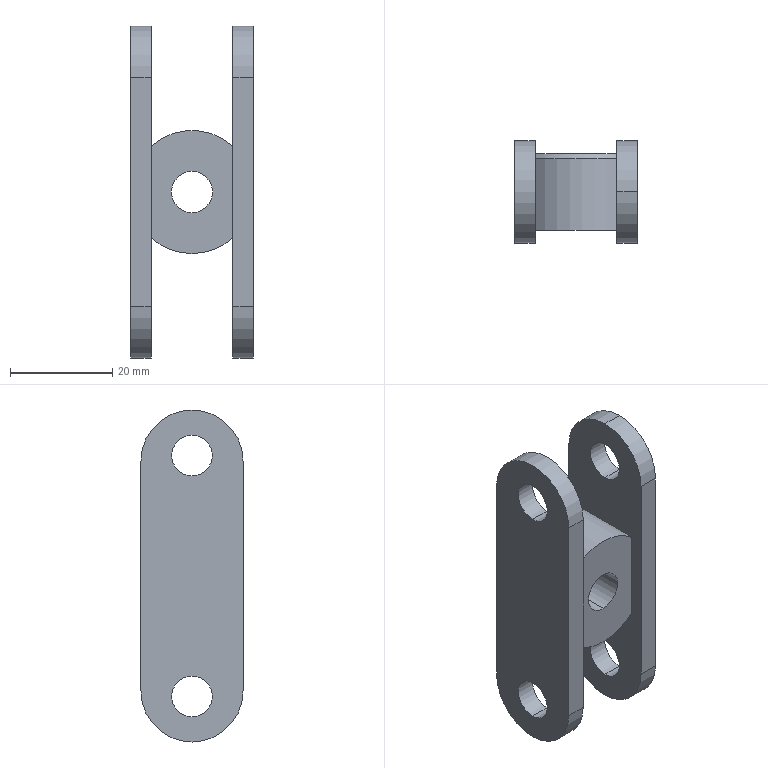Part | SolidWorks | features ICE 2, Chamfer 1, Extrusion 1, MirrorPattern 1 | 1 solid | 32 faces | box 24 x 20 x 65 mm | volume 13444 mm3 | cylinder 19 | plane 10 | cone 3 | commonest cylinder face diameters 8 x8 20 x6 24.1 x3 8.1 x2
STEP:
#1=CARTESIAN_POINT('',(-12.,7.5,27.58));
#2=VERTEX_POINT('',#1);
#3=CARTESIAN_POINT('',(-12.,7.5,19.58));
#4=VERTEX_POINT('',#3);
#5=CARTESIAN_POINT('',(-12.,7.5,23.58));
#6=DIRECTION('',(1.,0.,0.));
#7=DIRECTION('',(0.,0.,1.));
#8=AXIS2_PLACEMENT_3D('',#5,#6,#7);
#9=CIRCLE('',#8,4.);
#10=EDGE_CURVE('',#2,#4,#9,.T.);
#11=ORIENTED_EDGE('',*,*,#10,.F.);
#12=CARTESIAN_POINT('',(-8.,7.5,27.58));
#13=VERTEX_POINT('',#12);
#14=CARTESIAN_POINT('',(-12.,7.5,27.58));
#15=DIRECTION('',(1.,0.,0.));
#16=VECTOR('',#15,1000.);
#17=LINE('',#14,#16);
#18=EDGE_CURVE('',#2,#13,#17,.T.);
#19=ORIENTED_EDGE('',*,*,#18,.T.);
#20=CARTESIAN_POINT('',(-8.,7.5,19.58));
#21=VERTEX_POINT('',#20);
#22=CARTESIAN_POINT('',(-8.,7.5,23.58));
#23=DIRECTION('',(1.,0.,0.));
#24=DIRECTION('',(0.,0.,1.));
#25=AXIS2_PLACEMENT_3D('',#22,#23,#24);
#26=CIRCLE('',#25,4.);
#27=EDGE_CURVE('',#13,#21,#26,.T.);
#28=ORIENTED_EDGE('',*,*,#27,.T.);
#29=CARTESIAN_POINT('',(-12.,7.5,19.58));
#30=DIRECTION('',(1.,0.,0.));
#31=VECTOR('',#30,1000.);
#32=LINE('',#29,#31);
#33=EDGE_CURVE('',#4,#21,#32,.T.);
#34=ORIENTED_EDGE('',*,*,#33,.F.);
#35=EDGE_LOOP('',(#11,#19,#28,#34));
#36=FACE_OUTER_BOUND('',#35,.T.);
#37=CARTESIAN_POINT('',(-12.,7.5,23.58));
#38=DIRECTION('',(1.,0.,0.));
#39=DIRECTION('',(0.,0.,-1.));
#40=AXIS2_PLACEMENT_3D('',#37,#38,#39);
#41=CYLINDRICAL_SURFACE('',#40,4.);
#42=ADVANCED_FACE('',(#36),#41,.F.);
#43=CARTESIAN_POINT('',(-12.,7.5,-19.58));
#44=VERTEX_POINT('',#43);
#45=CARTESIAN_POINT('',(-12.,7.5,-27.58));
#46=VERTEX_POINT('',#45);
#47=CARTESIAN_POINT('',(-12.,7.5,-23.58));
#48=DIRECTION('',(1.,0.,0.));
#49=DIRECTION('',(0.,0.,-1.));
#50=AXIS2_PLACEMENT_3D('',#47,#48,#49);
#51=CIRCLE('',#50,4.);
#52=EDGE_CURVE('',#44,#46,#51,.T.);
#53=ORIENTED_EDGE('',*,*,#52,.F.);
#54=CARTESIAN_POINT('',(-8.,7.5,-19.58));
#55=VERTEX_POINT('',#54);
#56=CARTESIAN_POINT('',(-12.,7.5,-19.58));
#57=DIRECTION('',(1.,0.,0.));
#58=VECTOR('',#57,1000.);
#59=LINE('',#56,#58);
#60=EDGE_CURVE('',#44,#55,#59,.T.);
#61=ORIENTED_EDGE('',*,*,#60,.T.);
#62=CARTESIAN_POINT('',(-8.,7.5,-27.58));
#63=VERTEX_POINT('',#62);
#64=CARTESIAN_POINT('',(-8.,7.5,-23.58));
#65=DIRECTION('',(1.,0.,0.));
#66=DIRECTION('',(0.,0.,-1.));
#67=AXIS2_PLACEMENT_3D('',#64,#65,#66);
#68=CIRCLE('',#67,4.);
#69=EDGE_CURVE('',#55,#63,#68,.T.);
#70=ORIENTED_EDGE('',*,*,#69,.T.);
#71=CARTESIAN_POINT('',(-12.,7.5,-27.58));
#72=DIRECTION('',(1.,0.,0.));
#73=VECTOR('',#72,1000.);
#74=LINE('',#71,#73);
#75=EDGE_CURVE('',#46,#63,#74,.T.);
#76=ORIENTED_EDGE('',*,*,#75,.F.);
#77=EDGE_LOOP('',(#53,#61,#70,#76));
#78=FACE_OUTER_BOUND('',#77,.T.);
#79=CARTESIAN_POINT('',(-12.,7.5,-23.58));
#80=DIRECTION('',(1.,0.,0.));
#81=DIRECTION('',(0.,0.,-1.));
#82=AXIS2_PLACEMENT_3D('',#79,#80,#81);
#83=CYLINDRICAL_SURFACE('',#82,4.);
#84=ADVANCED_FACE('',(#78),#83,.F.);
#85=CARTESIAN_POINT('',(-12.,-2.5,-22.5));
#86=VERTEX_POINT('',#85);
#87=CARTESIAN_POINT('',(-12.,7.5,-32.5));
#88=VERTEX_POINT('',#87);
#89=CARTESIAN_POINT('',(-12.,7.5,-22.5));
#90=DIRECTION('',(1.,0.,0.));
#91=DIRECTION('',(0.,0.,-1.));
#92=AXIS2_PLACEMENT_3D('',#89,#90,#91);
#93=CIRCLE('',#92,10.);
#94=EDGE_CURVE('',#86,#88,#93,.T.);
#95=ORIENTED_EDGE('',*,*,#94,.T.);
#96=CARTESIAN_POINT('',(-8.,7.5,-32.5));
#97=VERTEX_POINT('',#96);
#98=CARTESIAN_POINT('',(-12.,7.5,-32.5));
#99=DIRECTION('',(1.,0.,0.));
#100=VECTOR('',#99,1000.);
#101=LINE('',#98,#100);
#102=EDGE_CURVE('',#88,#97,#101,.T.);
#103=ORIENTED_EDGE('',*,*,#102,.T.);
#104=CARTESIAN_POINT('',(-8.,-2.5,-22.5));
#105=VERTEX_POINT('',#104);
#106=CARTESIAN_POINT('',(-8.,7.5,-22.5));
#107=DIRECTION('',(1.,0.,0.));
#108=DIRECTION('',(0.,0.,-1.));
#109=AXIS2_PLACEMENT_3D('',#106,#107,#108);
#110=CIRCLE('',#109,10.);
#111=EDGE_CURVE('',#105,#97,#110,.T.);
#112=ORIENTED_EDGE('',*,*,#111,.F.);
#113=CARTESIAN_POINT('',(-12.,-2.5,-22.5));
#114=DIRECTION('',(1.,0.,0.));
#115=VECTOR('',#114,1000.);
#116=LINE('',#113,#115);
#117=EDGE_CURVE('',#86,#105,#116,.T.);
#118=ORIENTED_EDGE('',*,*,#117,.F.);
#119=EDGE_LOOP('',(#95,#103,#112,#118));
#120=FACE_OUTER_BOUND('',#119,.T.);
#121=CARTESIAN_POINT('',(-12.,7.5,-22.5));
#122=DIRECTION('',(1.,0.,0.));
#123=DIRECTION('',(0.,0.,-1.));
#124=AXIS2_PLACEMENT_3D('',#121,#122,#123);
#125=CYLINDRICAL_SURFACE('',#124,10.);
#126=ADVANCED_FACE('',(#120),#125,.T.);
#127=CARTESIAN_POINT('',(12.,7.5,27.58));
#128=VERTEX_POINT('',#127);
#129=CARTESIAN_POINT('',(12.,7.5,19.58));
#130=VERTEX_POINT('',#129);
#131=CARTESIAN_POINT('',(12.,7.5,23.58));
#132=DIRECTION('',(1.,0.,0.));
#133=DIRECTION('',(0.,0.,1.));
#134=AXIS2_PLACEMENT_3D('',#131,#132,#133);
#135=CIRCLE('',#134,4.);
#136=EDGE_CURVE('',#128,#130,#135,.T.);
#137=ORIENTED_EDGE('',*,*,#136,.T.);
#138=CARTESIAN_POINT('',(8.,7.5,19.58));
#139=VERTEX_POINT('',#138);
#140=CARTESIAN_POINT('',(12.,7.5,19.58));
#141=DIRECTION('',(-1.,0.,0.));
#142=VECTOR('',#141,1000.);
#143=LINE('',#140,#142);
#144=EDGE_CURVE('',#130,#139,#143,.T.);
#145=ORIENTED_EDGE('',*,*,#144,.T.);
#146=CARTESIAN_POINT('',(8.,7.5,27.58));
#147=VERTEX_POINT('',#146);
#148=CARTESIAN_POINT('',(8.,7.5,23.58));
#149=DIRECTION('',(1.,0.,0.));
#150=DIRECTION('',(0.,0.,1.));
#151=AXIS2_PLACEMENT_3D('',#148,#149,#150);
#152=CIRCLE('',#151,4.);
#153=EDGE_CURVE('',#147,#139,#152,.T.);
#154=ORIENTED_EDGE('',*,*,#153,.F.);
#155=CARTESIAN_POINT('',(12.,7.5,27.58));
#156=DIRECTION('',(-1.,0.,0.));
#157=VECTOR('',#156,1000.);
#158=LINE('',#155,#157);
#159=EDGE_CURVE('',#128,#147,#158,.T.);
#160=ORIENTED_EDGE('',*,*,#159,.F.);
#161=EDGE_LOOP('',(#137,#145,#154,#160));
#162=FACE_OUTER_BOUND('',#161,.T.);
#163=CARTESIAN_POINT('',(12.,7.5,23.58));
#164=DIRECTION('',(-1.,0.,0.));
#165=DIRECTION('',(0.,0.,1.));
#166=AXIS2_PLACEMENT_3D('',#163,#164,#165);
#167=CYLINDRICAL_SURFACE('',#166,4.);
#168=ADVANCED_FACE('',(#162),#167,.F.);
#169=CARTESIAN_POINT('',(12.,7.5,-19.58));
#170=VERTEX_POINT('',#169);
#171=CARTESIAN_POINT('',(12.,7.5,-27.58));
#172=VERTEX_POINT('',#171);
#173=CARTESIAN_POINT('',(12.,7.5,-23.58));
#174=DIRECTION('',(1.,0.,0.));
#175=DIRECTION('',(0.,0.,-1.));
#176=AXIS2_PLACEMENT_3D('',#173,#174,#175);
#177=CIRCLE('',#176,4.);
#178=EDGE_CURVE('',#170,#172,#177,.T.);
#179=ORIENTED_EDGE('',*,*,#178,.T.);
#180=CARTESIAN_POINT('',(8.,7.5,-27.58));
#181=VERTEX_POINT('',#180);
#182=CARTESIAN_POINT('',(12.,7.5,-27.58));
#183=DIRECTION('',(-1.,0.,0.));
#184=VECTOR('',#183,1000.);
#185=LINE('',#182,#184);
#186=EDGE_CURVE('',#172,#181,#185,.T.);
#187=ORIENTED_EDGE('',*,*,#186,.T.);
#188=CARTESIAN_POINT('',(8.,7.5,-19.58));
#189=VERTEX_POINT('',#188);
#190=CARTESIAN_POINT('',(8.,7.5,-23.58));
#191=DIRECTION('',(1.,0.,0.));
#192=DIRECTION('',(0.,0.,-1.));
#193=AXIS2_PLACEMENT_3D('',#190,#191,#192);
#194=CIRCLE('',#193,4.);
#195=EDGE_CURVE('',#189,#181,#194,.T.);
#196=ORIENTED_EDGE('',*,*,#195,.F.);
#197=CARTESIAN_POINT('',(12.,7.5,-19.58));
#198=DIRECTION('',(-1.,0.,0.));
#199=VECTOR('',#198,1000.);
#200=LINE('',#197,#199);
#201=EDGE_CURVE('',#170,#189,#200,.T.);
#202=ORIENTED_EDGE('',*,*,#201,.F.);
#203=EDGE_LOOP('',(#179,#187,#196,#202));
#204=FACE_OUTER_BOUND('',#203,.T.);
#205=CARTESIAN_POINT('',(12.,7.5,-23.58));
#206=DIRECTION('',(-1.,0.,0.));
#207=DIRECTION('',(0.,0.,1.));
#208=AXIS2_PLACEMENT_3D('',#205,#206,#207);
#209=CYLINDRICAL_SURFACE('',#208,4.);
#210=ADVANCED_FACE('',(#204),#209,.F.);
#211=CARTESIAN_POINT('',(12.,7.5,32.5));
#212=VERTEX_POINT('',#211);
#213=CARTESIAN_POINT('',(12.,-2.5,22.5));
#214=VERTEX_POINT('',#213);
#215=CARTESIAN_POINT('',(12.,7.5,22.5));
#216=DIRECTION('',(1.,0.,0.));
#217=DIRECTION('',(0.,0.,-1.));
#218=AXIS2_PLACEMENT_3D('',#215,#216,#217);
#219=CIRCLE('',#218,10.);
#220=EDGE_CURVE('',#212,#214,#219,.T.);
#221=ORIENTED_EDGE('',*,*,#220,.F.);
#222=CARTESIAN_POINT('',(8.,7.5,32.5));
#223=VERTEX_POINT('',#222);
#224=CARTESIAN_POINT('',(12.,7.5,32.5));
#225=DIRECTION('',(-1.,0.,0.));
#226=VECTOR('',#225,1000.);
#227=LINE('',#224,#226);
#228=EDGE_CURVE('',#212,#223,#227,.T.);
#229=ORIENTED_EDGE('',*,*,#228,.T.);
#230=CARTESIAN_POINT('',(8.,-2.5,22.5));
#231=VERTEX_POINT('',#230);
#232=CARTESIAN_POINT('',(8.,7.5,22.5));
#233=DIRECTION('',(1.,0.,0.));
#234=DIRECTION('',(0.,0.,-1.));
#235=AXIS2_PLACEMENT_3D('',#232,#233,#234);
#236=CIRCLE('',#235,10.);
#237=EDGE_CURVE('',#223,#231,#236,.T.);
#238=ORIENTED_EDGE('',*,*,#237,.T.);
#239=CARTESIAN_POINT('',(12.,-2.5,22.5));
#240=DIRECTION('',(-1.,0.,0.));
#241=VECTOR('',#240,1000.);
#242=LINE('',#239,#241);
#243=EDGE_CURVE('',#214,#231,#242,.T.);
#244=ORIENTED_EDGE('',*,*,#243,.F.);
#245=EDGE_LOOP('',(#221,#229,#238,#244));
#246=FACE_OUTER_BOUND('',#245,.T.);
#247=CARTESIAN_POINT('',(12.,7.5,22.5));
#248=DIRECTION('',(-1.,0.,0.));
#249=DIRECTION('',(0.,0.,1.));
#250=AXIS2_PLACEMENT_3D('',#247,#248,#249);
#251=CYLINDRICAL_SURFACE('',#250,10.);
#252=ADVANCED_FACE('',(#246),#251,.T.);
#253=CARTESIAN_POINT('',(0.,15.,-4.05));
#254=VERTEX_POINT('',#253);
#255=CARTESIAN_POINT('',(0.,15.,4.05));
#256=VERTEX_POINT('',#255);
#257=CARTESIAN_POINT('',(0.,15.,0.));
#258=DIRECTION('',(0.,1.,0.));
#259=DIRECTION('',(0.,0.,1.));
#260=AXIS2_PLACEMENT_3D('',#257,#258,#259);
#261=CIRCLE('',#260,4.05);
#262=EDGE_CURVE('',#254,#256,#261,.T.);
#263=ORIENTED_EDGE('',*,*,#262,.T.);
#264=CARTESIAN_POINT('',(0.,0.,4.05));
#265=VERTEX_POINT('',#264);
#266=CARTESIAN_POINT('',(0.,15.,4.05));
#267=DIRECTION('',(0.,-1.,0.));
#268=VECTOR('',#267,1000.);
#269=LINE('',#266,#268);
#270=EDGE_CURVE('',#256,#265,#269,.T.);
#271=ORIENTED_EDGE('',*,*,#270,.T.);
#272=CARTESIAN_POINT('',(0.,0.,-4.05));
#273=VERTEX_POINT('',#272);
#274=CARTESIAN_POINT('',(0.,0.,0.));
#275=DIRECTION('',(0.,1.,0.));
#276=DIRECTION('',(0.,0.,1.));
#277=AXIS2_PLACEMENT_3D('',#274,#275,#276);
#278=CIRCLE('',#277,4.05);
#279=EDGE_CURVE('',#273,#265,#278,.T.);
#280=ORIENTED_EDGE('',*,*,#279,.F.);
#281=CARTESIAN_POINT('',(0.,15.,-4.05));
#282=DIRECTION('',(0.,-1.,0.));
#283=VECTOR('',#282,1000.);
#284=LINE('',#281,#283);
#285=EDGE_CURVE('',#254,#273,#284,.T.);
#286=ORIENTED_EDGE('',*,*,#285,.F.);
#287=EDGE_LOOP('',(#263,#271,#280,#286));
#288=FACE_OUTER_BOUND('',#287,.T.);
#289=CARTESIAN_POINT('',(0.,15.,0.));
#290=DIRECTION('',(0.,-1.,0.));
#291=DIRECTION('',(0.,0.,-1.));
#292=AXIS2_PLACEMENT_3D('',#289,#290,#291);
#293=CYLINDRICAL_SURFACE('',#292,4.05);
#294=ADVANCED_FACE('',(#288),#293,.F.);
#295=CARTESIAN_POINT('',(0.,15.,-11.05));
#296=VERTEX_POINT('',#295);
#297=CARTESIAN_POINT('',(-8.,15.,-7.622));
#298=VERTEX_POINT('',#297);
#299=CARTESIAN_POINT('',(0.,15.,0.));
#300=DIRECTION('',(0.,1.,0.));
#301=DIRECTION('',(0.,0.,1.));
#302=AXIS2_PLACEMENT_3D('',#299,#300,#301);
#303=CIRCLE('',#302,11.05);
#304=EDGE_CURVE('',#296,#298,#303,.T.);
#305=ORIENTED_EDGE('',*,*,#304,.F.);
#306=CARTESIAN_POINT('',(0.,14.,-12.05));
#307=VERTEX_POINT('',#306);
#308=CARTESIAN_POINT('',(0.,15.,-11.05));
#309=DIRECTION('',(0.,-0.7071,-0.7071));
#310=VECTOR('',#309,1000.);
#311=LINE('',#308,#310);
#312=EDGE_CURVE('',#296,#307,#311,.T.);
#313=ORIENTED_EDGE('',*,*,#312,.T.);
#314=CARTESIAN_POINT('',(-8.,14.,-9.011));
#315=VERTEX_POINT('',#314);
#316=CARTESIAN_POINT('',(0.,14.,0.));
#317=DIRECTION('',(0.,-1.,0.));
#318=DIRECTION('',(0.,0.,1.));
#319=AXIS2_PLACEMENT_3D('',#316,#317,#318);
#320=CIRCLE('',#319,12.05);
#321=EDGE_CURVE('',#315,#307,#320,.T.);
#322=ORIENTED_EDGE('',*,*,#321,.F.);
#323=CARTESIAN_POINT('',(-8.,15.,-7.622));
#324=CARTESIAN_POINT('',(-8.,14.677,-8.091));
#325=CARTESIAN_POINT('',(-8.,14.342,-8.554));
#326=CARTESIAN_POINT('',(-8.,14.,-9.011));
#327=B_SPLINE_CURVE_WITH_KNOTS('',3,(#323,#324,#325,#326),.UNSPECIFIED.,.F.,.F.,(4,4),(0.0402,0.04192),.UNSPECIFIED.);
#328=EDGE_CURVE('',#298,#315,#327,.T.);
#329=ORIENTED_EDGE('',*,*,#328,.F.);
#330=EDGE_LOOP('',(#305,#313,#322,#329));
#331=FACE_OUTER_BOUND('',#330,.T.);
#332=CARTESIAN_POINT('',(0.,15.,0.));
#333=DIRECTION('',(0.,-1.,0.));
#334=DIRECTION('',(0.,0.,-1.));
#335=AXIS2_PLACEMENT_3D('',#332,#333,#334);
#336=CONICAL_SURFACE('',#335,11.05,0.7854);
#337=ADVANCED_FACE('',(#331),#336,.T.);
#338=ORIENTED_EDGE('',*,*,#321,.T.);
#339=CARTESIAN_POINT('',(0.,0.,-12.05));
#340=VERTEX_POINT('',#339);
#341=CARTESIAN_POINT('',(0.,15.,-12.05));
#342=DIRECTION('',(0.,-1.,0.));
#343=VECTOR('',#342,1000.);
#344=LINE('',#341,#343);
#345=EDGE_CURVE('',#307,#340,#344,.T.);
#346=ORIENTED_EDGE('',*,*,#345,.T.);
#347=CARTESIAN_POINT('',(-8.,0.,-9.011));
#348=VERTEX_POINT('',#347);
#349=CARTESIAN_POINT('',(0.,0.,0.));
#350=DIRECTION('',(0.,1.,0.));
#351=DIRECTION('',(0.,0.,1.));
#352=AXIS2_PLACEMENT_3D('',#349,#350,#351);
#353=CIRCLE('',#352,12.05);
#354=EDGE_CURVE('',#340,#348,#353,.T.);
#355=ORIENTED_EDGE('',*,*,#354,.T.);
#356=CARTESIAN_POINT('',(-8.,15.,-9.011));
#357=DIRECTION('',(0.,1.,0.));
#358=VECTOR('',#357,1000.);
#359=LINE('',#356,#358);
#360=EDGE_CURVE('',#348,#315,#359,.T.);
#361=ORIENTED_EDGE('',*,*,#360,.T.);
#362=EDGE_LOOP('',(#338,#346,#355,#361));
#363=FACE_OUTER_BOUND('',#362,.T.);
#364=CARTESIAN_POINT('',(0.,15.,0.));
#365=DIRECTION('',(0.,-1.,0.));
#366=DIRECTION('',(0.,0.,-1.));
#367=AXIS2_PLACEMENT_3D('',#364,#365,#366);
#368=CYLINDRICAL_SURFACE('',#367,12.05);
#369=ADVANCED_FACE('',(#363),#368,.T.);
#370=ORIENTED_EDGE('',*,*,#345,.F.);
#371=CARTESIAN_POINT('',(8.,14.,-9.011));
#372=VERTEX_POINT('',#371);
#373=CARTESIAN_POINT('',(0.,14.,0.));
#374=DIRECTION('',(0.,-1.,0.));
#375=DIRECTION('',(0.,0.,1.));
#376=AXIS2_PLACEMENT_3D('',#373,#374,#375);
#377=CIRCLE('',#376,12.05);
#378=EDGE_CURVE('',#307,#372,#377,.T.);
#379=ORIENTED_EDGE('',*,*,#378,.T.);
#380=CARTESIAN_POINT('',(8.,0.,-9.011));
#381=VERTEX_POINT('',#380);
#382=CARTESIAN_POINT('',(8.,15.,-9.011));
#383=DIRECTION('',(0.,1.,0.));
#384=VECTOR('',#383,1000.);
#385=LINE('',#382,#384);
#386=EDGE_CURVE('',#381,#372,#385,.T.);
#387=ORIENTED_EDGE('',*,*,#386,.F.);
#388=CARTESIAN_POINT('',(0.,0.,0.));
#389=DIRECTION('',(0.,1.,0.));
#390=DIRECTION('',(0.,0.,1.));
#391=AXIS2_PLACEMENT_3D('',#388,#389,#390);
#392=CIRCLE('',#391,12.05);
#393=EDGE_CURVE('',#381,#340,#392,.T.);
#394=ORIENTED_EDGE('',*,*,#393,.T.);
#395=EDGE_LOOP('',(#370,#379,#387,#394));
#396=FACE_OUTER_BOUND('',#395,.T.);
#397=CARTESIAN_POINT('',(0.,15.,0.));
#398=DIRECTION('',(0.,-1.,0.));
#399=DIRECTION('',(0.,0.,-1.));
#400=AXIS2_PLACEMENT_3D('',#397,#398,#399);
#401=CYLINDRICAL_SURFACE('',#400,12.05);
#402=ADVANCED_FACE('',(#396),#401,.T.);
#403=ORIENTED_EDGE('',*,*,#312,.F.);
#404=CARTESIAN_POINT('',(8.,15.,-7.622));
#405=VERTEX_POINT('',#404);
#406=CARTESIAN_POINT('',(0.,15.,0.));
#407=DIRECTION('',(0.,1.,0.));
#408=DIRECTION('',(0.,0.,1.));
#409=AXIS2_PLACEMENT_3D('',#406,#407,#408);
#410=CIRCLE('',#409,11.05);
#411=EDGE_CURVE('',#405,#296,#410,.T.);
#412=ORIENTED_EDGE('',*,*,#411,.F.);
#413=CARTESIAN_POINT('',(8.,15.,-7.622));
#414=CARTESIAN_POINT('',(8.,14.677,-8.091));
#415=CARTESIAN_POINT('',(8.,14.342,-8.554));
#416=CARTESIAN_POINT('',(8.,14.,-9.011));
#417=B_SPLINE_CURVE_WITH_KNOTS('',3,(#413,#414,#415,#416),.UNSPECIFIED.,.F.,.F.,(4,4),(0.0402,0.04192),.UNSPECIFIED.);
#418=EDGE_CURVE('',#405,#372,#417,.T.);
#419=ORIENTED_EDGE('',*,*,#418,.T.);
#420=ORIENTED_EDGE('',*,*,#378,.F.);
#421=EDGE_LOOP('',(#403,#412,#419,#420));
#422=FACE_OUTER_BOUND('',#421,.T.);
#423=CARTESIAN_POINT('',(0.,15.,0.));
#424=DIRECTION('',(0.,-1.,0.));
#425=DIRECTION('',(0.,0.,-1.));
#426=AXIS2_PLACEMENT_3D('',#423,#424,#425);
#427=CONICAL_SURFACE('',#426,11.05,0.7854);
#428=ADVANCED_FACE('',(#422),#427,.T.);
#429=CARTESIAN_POINT('',(8.,15.,7.622));
#430=VERTEX_POINT('',#429);
#431=CARTESIAN_POINT('',(8.,15.,-18.778));
#432=DIRECTION('',(0.,0.,1.));
#433=VECTOR('',#432,1000.);
#434=LINE('',#431,#433);
#435=EDGE_CURVE('',#405,#430,#434,.T.);
#436=ORIENTED_EDGE('',*,*,#435,.F.);
#437=ORIENTED_EDGE('',*,*,#411,.T.);
#438=ORIENTED_EDGE('',*,*,#304,.T.);
#439=CARTESIAN_POINT('',(-8.,15.,7.622));
#440=VERTEX_POINT('',#439);
#441=CARTESIAN_POINT('',(-8.,15.,-18.778));
#442=DIRECTION('',(0.,0.,1.));
#443=VECTOR('',#442,1000.);
#444=LINE('',#441,#443);
#445=EDGE_CURVE('',#298,#440,#444,.T.);
#446=ORIENTED_EDGE('',*,*,#445,.T.);
#447=CARTESIAN_POINT('',(0.,15.,0.));
#448=DIRECTION('',(0.,1.,0.));
#449=DIRECTION('',(0.,0.,1.));
#450=AXIS2_PLACEMENT_3D('',#447,#448,#449);
#451=CIRCLE('',#450,11.05);
#452=EDGE_CURVE('',#440,#430,#451,.T.);
#453=ORIENTED_EDGE('',*,*,#452,.T.);
#454=EDGE_LOOP('',(#436,#437,#438,#446,#453));
#455=FACE_OUTER_BOUND('',#454,.T.);
#456=ORIENTED_EDGE('',*,*,#262,.F.);
#457=CARTESIAN_POINT('',(0.,15.,0.));
#458=DIRECTION('',(0.,1.,0.));
#459=DIRECTION('',(0.,0.,1.));
#460=AXIS2_PLACEMENT_3D('',#457,#458,#459);
#461=CIRCLE('',#460,4.05);
#462=EDGE_CURVE('',#256,#254,#461,.T.);
#463=ORIENTED_EDGE('',*,*,#462,.F.);
#464=EDGE_LOOP('',(#456,#463));
#465=FACE_BOUND('',#464,.T.);
#466=CARTESIAN_POINT('',(0.,15.,0.));
#467=DIRECTION('',(0.,1.,0.));
#468=DIRECTION('',(0.,0.,1.));
#469=AXIS2_PLACEMENT_3D('',#466,#467,#468);
#470=PLANE('',#469);
#471=ADVANCED_FACE('',(#455,#465),#470,.T.);
#472=ORIENTED_EDGE('',*,*,#279,.T.);
#473=CARTESIAN_POINT('',(0.,0.,0.));
#474=DIRECTION('',(0.,1.,0.));
#475=DIRECTION('',(0.,0.,1.));
#476=AXIS2_PLACEMENT_3D('',#473,#474,#475);
#477=CIRCLE('',#476,4.05);
#478=EDGE_CURVE('',#265,#273,#477,.T.);
#479=ORIENTED_EDGE('',*,*,#478,.T.);
#480=EDGE_LOOP('',(#472,#479));
#481=FACE_BOUND('',#480,.T.);
#482=ORIENTED_EDGE('',*,*,#393,.F.);
#483=CARTESIAN_POINT('',(8.,0.,9.011));
#484=VERTEX_POINT('',#483);
#485=CARTESIAN_POINT('',(8.,0.,-18.778));
#486=DIRECTION('',(0.,0.,-1.));
#487=VECTOR('',#486,1000.);
#488=LINE('',#485,#487);
#489=EDGE_CURVE('',#484,#381,#488,.T.);
#490=ORIENTED_EDGE('',*,*,#489,.F.);
#491=CARTESIAN_POINT('',(-8.,0.,9.011));
#492=VERTEX_POINT('',#491);
#493=CARTESIAN_POINT('',(0.,0.,0.));
#494=DIRECTION('',(0.,1.,0.));
#495=DIRECTION('',(0.,0.,1.));
#496=AXIS2_PLACEMENT_3D('',#493,#494,#495);
#497=CIRCLE('',#496,12.05);
#498=EDGE_CURVE('',#492,#484,#497,.T.);
#499=ORIENTED_EDGE('',*,*,#498,.F.);
#500=CARTESIAN_POINT('',(-8.,0.,-18.778));
#501=DIRECTION('',(0.,0.,-1.));
#502=VECTOR('',#501,1000.);
#503=LINE('',#500,#502);
#504=EDGE_CURVE('',#492,#348,#503,.T.);
#505=ORIENTED_EDGE('',*,*,#504,.T.);
#506=ORIENTED_EDGE('',*,*,#354,.F.);
#507=EDGE_LOOP('',(#482,#490,#499,#505,#506));
#508=FACE_OUTER_BOUND('',#507,.T.);
#509=CARTESIAN_POINT('',(0.,0.,0.));
#510=DIRECTION('',(0.,1.,0.));
#511=DIRECTION('',(0.,0.,1.));
#512=AXIS2_PLACEMENT_3D('',#509,#510,#511);
#513=PLANE('',#512);
#514=ADVANCED_FACE('',(#481,#508),#513,.F.);
#515=ORIENTED_EDGE('',*,*,#498,.T.);
#516=CARTESIAN_POINT('',(8.,14.,9.011));
#517=VERTEX_POINT('',#516);
#518=CARTESIAN_POINT('',(8.,15.,9.011));
#519=DIRECTION('',(0.,-1.,0.));
#520=VECTOR('',#519,1000.);
#521=LINE('',#518,#520);
#522=EDGE_CURVE('',#517,#484,#521,.T.);
#523=ORIENTED_EDGE('',*,*,#522,.F.);
#524=CARTESIAN_POINT('',(-8.,14.,9.011));
#525=VERTEX_POINT('',#524);
#526=CARTESIAN_POINT('',(0.,14.,0.));
#527=DIRECTION('',(0.,-1.,0.));
#528=DIRECTION('',(0.,0.,1.));
#529=AXIS2_PLACEMENT_3D('',#526,#527,#528);
#530=CIRCLE('',#529,12.05);
#531=EDGE_CURVE('',#517,#525,#530,.T.);
#532=ORIENTED_EDGE('',*,*,#531,.T.);
#533=CARTESIAN_POINT('',(-8.,15.,9.011));
#534=DIRECTION('',(0.,-1.,0.));
#535=VECTOR('',#534,1000.);
#536=LINE('',#533,#535);
#537=EDGE_CURVE('',#525,#492,#536,.T.);
#538=ORIENTED_EDGE('',*,*,#537,.T.);
#539=EDGE_LOOP('',(#515,#523,#532,#538));
#540=FACE_OUTER_BOUND('',#539,.T.);
#541=CARTESIAN_POINT('',(0.,15.,0.));
#542=DIRECTION('',(0.,-1.,0.));
#543=DIRECTION('',(0.,0.,-1.));
#544=AXIS2_PLACEMENT_3D('',#541,#542,#543);
#545=CYLINDRICAL_SURFACE('',#544,12.05);
#546=ADVANCED_FACE('',(#540),#545,.T.);
#547=CARTESIAN_POINT('',(8.,14.,9.011));
#548=CARTESIAN_POINT('',(8.,14.341,8.555));
#549=CARTESIAN_POINT('',(8.,14.676,8.093));
#550=CARTESIAN_POINT('',(8.,15.,7.622));
#551=B_SPLINE_CURVE_WITH_KNOTS('',3,(#547,#548,#549,#550),.UNSPECIFIED.,.F.,.F.,(4,4),(0.02179,0.02351),.UNSPECIFIED.);
#552=EDGE_CURVE('',#517,#430,#551,.T.);
#553=ORIENTED_EDGE('',*,*,#552,.T.);
#554=ORIENTED_EDGE('',*,*,#452,.F.);
#555=CARTESIAN_POINT('',(-8.,14.,9.011));
#556=CARTESIAN_POINT('',(-8.,14.341,8.555));
#557=CARTESIAN_POINT('',(-8.,14.676,8.093));
#558=CARTESIAN_POINT('',(-8.,15.,7.622));
#559=B_SPLINE_CURVE_WITH_KNOTS('',3,(#555,#556,#557,#558),.UNSPECIFIED.,.F.,.F.,(4,4),(0.02179,0.02351),.UNSPECIFIED.);
#560=EDGE_CURVE('',#525,#440,#559,.T.);
#561=ORIENTED_EDGE('',*,*,#560,.F.);
#562=ORIENTED_EDGE('',*,*,#531,.F.);
#563=EDGE_LOOP('',(#553,#554,#561,#562));
#564=FACE_OUTER_BOUND('',#563,.T.);
#565=CARTESIAN_POINT('',(0.,15.,0.));
#566=DIRECTION('',(0.,-1.,0.));
#567=DIRECTION('',(0.,0.,-1.));
#568=AXIS2_PLACEMENT_3D('',#565,#566,#567);
#569=CONICAL_SURFACE('',#568,11.05,0.7854);
#570=ADVANCED_FACE('',(#564),#569,.T.);
#571=ORIENTED_EDGE('',*,*,#270,.F.);
#572=ORIENTED_EDGE('',*,*,#462,.T.);
#573=ORIENTED_EDGE('',*,*,#285,.T.);
#574=ORIENTED_EDGE('',*,*,#478,.F.);
#575=EDGE_LOOP('',(#571,#572,#573,#574));
#576=FACE_OUTER_BOUND('',#575,.T.);
#577=CARTESIAN_POINT('',(0.,15.,0.));
#578=DIRECTION('',(0.,-1.,0.));
#579=DIRECTION('',(0.,0.,-1.));
#580=AXIS2_PLACEMENT_3D('',#577,#578,#579);
#581=CYLINDRICAL_SURFACE('',#580,4.05);
#582=ADVANCED_FACE('',(#576),#581,.F.);
#583=CARTESIAN_POINT('',(8.,-2.5,-22.5));
#584=VERTEX_POINT('',#583);
#585=CARTESIAN_POINT('',(8.,17.5,-22.5));
#586=VERTEX_POINT('',#585);
#587=CARTESIAN_POINT('',(8.,7.5,-22.5));
#588=DIRECTION('',(1.,0.,0.));
#589=DIRECTION('',(0.,0.,-1.));
#590=AXIS2_PLACEMENT_3D('',#587,#588,#589);
#591=CIRCLE('',#590,10.);
#592=EDGE_CURVE('',#584,#586,#591,.T.);
#593=ORIENTED_EDGE('',*,*,#592,.F.);
#594=CARTESIAN_POINT('',(8.,-2.5,-22.5));
#595=DIRECTION('',(0.,0.,-1.));
#596=VECTOR('',#595,1000.);
#597=LINE('',#594,#596);
#598=EDGE_CURVE('',#231,#584,#597,.T.);
#599=ORIENTED_EDGE('',*,*,#598,.F.);
#600=ORIENTED_EDGE('',*,*,#237,.F.);
#601=CARTESIAN_POINT('',(8.,17.5,22.5));
#602=VERTEX_POINT('',#601);
#603=CARTESIAN_POINT('',(8.,7.5,22.5));
#604=DIRECTION('',(1.,0.,0.));
#605=DIRECTION('',(0.,0.,-1.));
#606=AXIS2_PLACEMENT_3D('',#603,#604,#605);
#607=CIRCLE('',#606,10.);
#608=EDGE_CURVE('',#602,#223,#607,.T.);
#609=ORIENTED_EDGE('',*,*,#608,.F.);
#610=CARTESIAN_POINT('',(8.,17.5,-22.5));
#611=DIRECTION('',(0.,0.,1.));
#612=VECTOR('',#611,1000.);
#613=LINE('',#610,#612);
#614=EDGE_CURVE('',#586,#602,#613,.T.);
#615=ORIENTED_EDGE('',*,*,#614,.F.);
#616=EDGE_LOOP('',(#593,#599,#600,#609,#615));
#617=FACE_OUTER_BOUND('',#616,.T.);
#618=ORIENTED_EDGE('',*,*,#195,.T.);
#619=CARTESIAN_POINT('',(8.,7.5,-23.58));
#620=DIRECTION('',(1.,0.,0.));
#621=DIRECTION('',(0.,0.,-1.));
#622=AXIS2_PLACEMENT_3D('',#619,#620,#621);
#623=CIRCLE('',#622,4.);
#624=EDGE_CURVE('',#181,#189,#623,.T.);
#625=ORIENTED_EDGE('',*,*,#624,.T.);
#626=EDGE_LOOP('',(#618,#625));
#627=FACE_BOUND('',#626,.T.);
#628=ORIENTED_EDGE('',*,*,#153,.T.);
#629=CARTESIAN_POINT('',(8.,7.5,23.58));
#630=DIRECTION('',(1.,0.,0.));
#631=DIRECTION('',(0.,0.,1.));
#632=AXIS2_PLACEMENT_3D('',#629,#630,#631);
#633=CIRCLE('',#632,4.);
#634=EDGE_CURVE('',#139,#147,#633,.T.);
#635=ORIENTED_EDGE('',*,*,#634,.T.);
#636=EDGE_LOOP('',(#628,#635));
#637=FACE_BOUND('',#636,.T.);
#638=ORIENTED_EDGE('',*,*,#489,.T.);
#639=ORIENTED_EDGE('',*,*,#386,.T.);
#640=ORIENTED_EDGE('',*,*,#418,.F.);
#641=ORIENTED_EDGE('',*,*,#435,.T.);
#642=ORIENTED_EDGE('',*,*,#552,.F.);
#643=ORIENTED_EDGE('',*,*,#522,.T.);
#644=EDGE_LOOP('',(#638,#639,#640,#641,#642,#643));
#645=FACE_BOUND('',#644,.T.);
#646=CARTESIAN_POINT('',(8.,7.5,-22.5));
#647=DIRECTION('',(1.,0.,0.));
#648=DIRECTION('',(0.,0.,-1.));
#649=AXIS2_PLACEMENT_3D('',#646,#647,#648);
#650=PLANE('',#649);
#651=ADVANCED_FACE('',(#617,#627,#637,#645),#650,.F.);
#652=ORIENTED_EDGE('',*,*,#178,.F.);
#653=CARTESIAN_POINT('',(12.,7.5,-23.58));
#654=DIRECTION('',(1.,0.,0.));
#655=DIRECTION('',(0.,0.,-1.));
#656=AXIS2_PLACEMENT_3D('',#653,#654,#655);
#657=CIRCLE('',#656,4.);
#658=EDGE_CURVE('',#172,#170,#657,.T.);
#659=ORIENTED_EDGE('',*,*,#658,.F.);
#660=EDGE_LOOP('',(#652,#659));
#661=FACE_BOUND('',#660,.T.);
#662=CARTESIAN_POINT('',(12.,-2.5,-22.5));
#663=VERTEX_POINT('',#662);
#664=CARTESIAN_POINT('',(12.,17.5,-22.5));
#665=VERTEX_POINT('',#664);
#666=CARTESIAN_POINT('',(12.,7.5,-22.5));
#667=DIRECTION('',(1.,0.,0.));
#668=DIRECTION('',(0.,0.,-1.));
#669=AXIS2_PLACEMENT_3D('',#666,#667,#668);
#670=CIRCLE('',#669,10.);
#671=EDGE_CURVE('',#663,#665,#670,.T.);
#672=ORIENTED_EDGE('',*,*,#671,.T.);
#673=CARTESIAN_POINT('',(12.,17.5,22.5));
#674=VERTEX_POINT('',#673);
#675=CARTESIAN_POINT('',(12.,17.5,-22.5));
#676=DIRECTION('',(0.,0.,1.));
#677=VECTOR('',#676,1000.);
#678=LINE('',#675,#677);
#679=EDGE_CURVE('',#665,#674,#678,.T.);
#680=ORIENTED_EDGE('',*,*,#679,.T.);
#681=CARTESIAN_POINT('',(12.,7.5,22.5));
#682=DIRECTION('',(1.,0.,0.));
#683=DIRECTION('',(0.,0.,-1.));
#684=AXIS2_PLACEMENT_3D('',#681,#682,#683);
#685=CIRCLE('',#684,10.);
#686=EDGE_CURVE('',#674,#212,#685,.T.);
#687=ORIENTED_EDGE('',*,*,#686,.T.);
#688=ORIENTED_EDGE('',*,*,#220,.T.);
#689=CARTESIAN_POINT('',(12.,-2.5,-22.5));
#690=DIRECTION('',(0.,0.,-1.));
#691=VECTOR('',#690,1000.);
#692=LINE('',#689,#691);
#693=EDGE_CURVE('',#214,#663,#692,.T.);
#694=ORIENTED_EDGE('',*,*,#693,.T.);
#695=EDGE_LOOP('',(#672,#680,#687,#688,#694));
#696=FACE_OUTER_BOUND('',#695,.T.);
#697=ORIENTED_EDGE('',*,*,#136,.F.);
#698=CARTESIAN_POINT('',(12.,7.5,23.58));
#699=DIRECTION('',(1.,0.,0.));
#700=DIRECTION('',(0.,0.,1.));
#701=AXIS2_PLACEMENT_3D('',#698,#699,#700);
#702=CIRCLE('',#701,4.);
#703=EDGE_CURVE('',#130,#128,#702,.T.);
#704=ORIENTED_EDGE('',*,*,#703,.F.);
#705=EDGE_LOOP('',(#697,#704));
#706=FACE_BOUND('',#705,.T.);
#707=CARTESIAN_POINT('',(12.,7.5,-22.5));
#708=DIRECTION('',(1.,0.,0.));
#709=DIRECTION('',(0.,0.,-1.));
#710=AXIS2_PLACEMENT_3D('',#707,#708,#709);
#711=PLANE('',#710);
#712=ADVANCED_FACE('',(#661,#696,#706),#711,.T.);
#713=ORIENTED_EDGE('',*,*,#592,.T.);
#714=CARTESIAN_POINT('',(12.,17.5,-22.5));
#715=DIRECTION('',(-1.,0.,0.));
#716=VECTOR('',#715,1000.);
#717=LINE('',#714,#716);
#718=EDGE_CURVE('',#665,#586,#717,.T.);
#719=ORIENTED_EDGE('',*,*,#718,.F.);
#720=ORIENTED_EDGE('',*,*,#671,.F.);
#721=CARTESIAN_POINT('',(12.,-2.5,-22.5));
#722=DIRECTION('',(-1.,0.,0.));
#723=VECTOR('',#722,1000.);
#724=LINE('',#721,#723);
#725=EDGE_CURVE('',#663,#584,#724,.T.);
#726=ORIENTED_EDGE('',*,*,#725,.T.);
#727=EDGE_LOOP('',(#713,#719,#720,#726));
#728=FACE_OUTER_BOUND('',#727,.T.);
#729=CARTESIAN_POINT('',(12.,7.5,-22.5));
#730=DIRECTION('',(-1.,0.,0.));
#731=DIRECTION('',(0.,0.,1.));
#732=AXIS2_PLACEMENT_3D('',#729,#730,#731);
#733=CYLINDRICAL_SURFACE('',#732,10.);
#734=ADVANCED_FACE('',(#728),#733,.T.);
#735=ORIENTED_EDGE('',*,*,#614,.T.);
#736=CARTESIAN_POINT('',(12.,17.5,22.5));
#737=DIRECTION('',(-1.,0.,0.));
#738=VECTOR('',#737,1000.);
#739=LINE('',#736,#738);
#740=EDGE_CURVE('',#674,#602,#739,.T.);
#741=ORIENTED_EDGE('',*,*,#740,.F.);
#742=ORIENTED_EDGE('',*,*,#679,.F.);
#743=ORIENTED_EDGE('',*,*,#718,.T.);
#744=EDGE_LOOP('',(#735,#741,#742,#743));
#745=FACE_OUTER_BOUND('',#744,.T.);
#746=CARTESIAN_POINT('',(12.,17.5,-22.5));
#747=DIRECTION('',(0.,-1.,0.));
#748=DIRECTION('',(0.,0.,-1.));
#749=AXIS2_PLACEMENT_3D('',#746,#747,#748);
#750=PLANE('',#749);
#751=ADVANCED_FACE('',(#745),#750,.F.);
#752=ORIENTED_EDGE('',*,*,#228,.F.);
#753=ORIENTED_EDGE('',*,*,#686,.F.);
#754=ORIENTED_EDGE('',*,*,#740,.T.);
#755=ORIENTED_EDGE('',*,*,#608,.T.);
#756=EDGE_LOOP('',(#752,#753,#754,#755));
#757=FACE_OUTER_BOUND('',#756,.T.);
#758=CARTESIAN_POINT('',(12.,7.5,22.5));
#759=DIRECTION('',(-1.,0.,0.));
#760=DIRECTION('',(0.,0.,1.));
#761=AXIS2_PLACEMENT_3D('',#758,#759,#760);
#762=CYLINDRICAL_SURFACE('',#761,10.);
#763=ADVANCED_FACE('',(#757),#762,.T.);
#764=ORIENTED_EDGE('',*,*,#598,.T.);
#765=ORIENTED_EDGE('',*,*,#725,.F.);
#766=ORIENTED_EDGE('',*,*,#693,.F.);
#767=ORIENTED_EDGE('',*,*,#243,.T.);
#768=EDGE_LOOP('',(#764,#765,#766,#767));
#769=FACE_OUTER_BOUND('',#768,.T.);
#770=CARTESIAN_POINT('',(12.,-2.5,-22.5));
#771=DIRECTION('',(0.,1.,0.));
#772=DIRECTION('',(0.,0.,1.));
#773=AXIS2_PLACEMENT_3D('',#770,#771,#772);
#774=PLANE('',#773);
#775=ADVANCED_FACE('',(#769),#774,.F.);
#776=ORIENTED_EDGE('',*,*,#186,.F.);
#777=ORIENTED_EDGE('',*,*,#658,.T.);
#778=ORIENTED_EDGE('',*,*,#201,.T.);
#779=ORIENTED_EDGE('',*,*,#624,.F.);
#780=EDGE_LOOP('',(#776,#777,#778,#779));
#781=FACE_OUTER_BOUND('',#780,.T.);
#782=CARTESIAN_POINT('',(12.,7.5,-23.58));
#783=DIRECTION('',(-1.,0.,0.));
#784=DIRECTION('',(0.,0.,1.));
#785=AXIS2_PLACEMENT_3D('',#782,#783,#784);
#786=CYLINDRICAL_SURFACE('',#785,4.);
#787=ADVANCED_FACE('',(#781),#786,.F.);
#788=ORIENTED_EDGE('',*,*,#144,.F.);
#789=ORIENTED_EDGE('',*,*,#703,.T.);
#790=ORIENTED_EDGE('',*,*,#159,.T.);
#791=ORIENTED_EDGE('',*,*,#634,.F.);
#792=EDGE_LOOP('',(#788,#789,#790,#791));
#793=FACE_OUTER_BOUND('',#792,.T.);
#794=CARTESIAN_POINT('',(12.,7.5,23.58));
#795=DIRECTION('',(-1.,0.,0.));
#796=DIRECTION('',(0.,0.,1.));
#797=AXIS2_PLACEMENT_3D('',#794,#795,#796);
#798=CYLINDRICAL_SURFACE('',#797,4.);
#799=ADVANCED_FACE('',(#793),#798,.F.);
#800=CARTESIAN_POINT('',(-8.,7.5,23.58));
#801=DIRECTION('',(1.,0.,0.));
#802=DIRECTION('',(0.,0.,1.));
#803=AXIS2_PLACEMENT_3D('',#800,#801,#802);
#804=CIRCLE('',#803,4.);
#805=EDGE_CURVE('',#21,#13,#804,.T.);
#806=ORIENTED_EDGE('',*,*,#805,.F.);
#807=ORIENTED_EDGE('',*,*,#27,.F.);
#808=EDGE_LOOP('',(#806,#807));
#809=FACE_BOUND('',#808,.T.);
#810=CARTESIAN_POINT('',(-8.,7.5,-23.58));
#811=DIRECTION('',(1.,0.,0.));
#812=DIRECTION('',(0.,0.,-1.));
#813=AXIS2_PLACEMENT_3D('',#810,#811,#812);
#814=CIRCLE('',#813,4.);
#815=EDGE_CURVE('',#63,#55,#814,.T.);
#816=ORIENTED_EDGE('',*,*,#815,.F.);
#817=ORIENTED_EDGE('',*,*,#69,.F.);
#818=EDGE_LOOP('',(#816,#817));
#819=FACE_BOUND('',#818,.T.);
#820=ORIENTED_EDGE('',*,*,#111,.T.);
#821=CARTESIAN_POINT('',(-8.,17.5,-22.5));
#822=VERTEX_POINT('',#821);
#823=CARTESIAN_POINT('',(-8.,7.5,-22.5));
#824=DIRECTION('',(1.,0.,0.));
#825=DIRECTION('',(0.,0.,-1.));
#826=AXIS2_PLACEMENT_3D('',#823,#824,#825);
#827=CIRCLE('',#826,10.);
#828=EDGE_CURVE('',#97,#822,#827,.T.);
#829=ORIENTED_EDGE('',*,*,#828,.T.);
#830=CARTESIAN_POINT('',(-8.,17.5,22.5));
#831=VERTEX_POINT('',#830);
#832=CARTESIAN_POINT('',(-8.,17.5,-22.5));
#833=DIRECTION('',(0.,0.,1.));
#834=VECTOR('',#833,1000.);
#835=LINE('',#832,#834);
#836=EDGE_CURVE('',#822,#831,#835,.T.);
#837=ORIENTED_EDGE('',*,*,#836,.T.);
#838=CARTESIAN_POINT('',(-8.,-2.5,22.5));
#839=VERTEX_POINT('',#838);
#840=CARTESIAN_POINT('',(-8.,7.5,22.5));
#841=DIRECTION('',(1.,0.,0.));
#842=DIRECTION('',(0.,0.,-1.));
#843=AXIS2_PLACEMENT_3D('',#840,#841,#842);
#844=CIRCLE('',#843,10.);
#845=EDGE_CURVE('',#831,#839,#844,.T.);
#846=ORIENTED_EDGE('',*,*,#845,.T.);
#847=CARTESIAN_POINT('',(-8.,-2.5,-22.5));
#848=DIRECTION('',(0.,0.,-1.));
#849=VECTOR('',#848,1000.);
#850=LINE('',#847,#849);
#851=EDGE_CURVE('',#839,#105,#850,.T.);
#852=ORIENTED_EDGE('',*,*,#851,.T.);
#853=EDGE_LOOP('',(#820,#829,#837,#846,#852));
#854=FACE_OUTER_BOUND('',#853,.T.);
#855=ORIENTED_EDGE('',*,*,#328,.T.);
#856=ORIENTED_EDGE('',*,*,#360,.F.);
#857=ORIENTED_EDGE('',*,*,#504,.F.);
#858=ORIENTED_EDGE('',*,*,#537,.F.);
#859=ORIENTED_EDGE('',*,*,#560,.T.);
#860=ORIENTED_EDGE('',*,*,#445,.F.);
#861=EDGE_LOOP('',(#855,#856,#857,#858,#859,#860));
#862=FACE_BOUND('',#861,.T.);
#863=CARTESIAN_POINT('',(-8.,7.5,-22.5));
#864=DIRECTION('',(-1.,0.,0.));
#865=DIRECTION('',(0.,0.,-1.));
#866=AXIS2_PLACEMENT_3D('',#863,#864,#865);
#867=PLANE('',#866);
#868=ADVANCED_FACE('',(#809,#819,#854,#862),#867,.F.);
#869=ORIENTED_EDGE('',*,*,#102,.F.);
#870=CARTESIAN_POINT('',(-12.,17.5,-22.5));
#871=VERTEX_POINT('',#870);
#872=CARTESIAN_POINT('',(-12.,7.5,-22.5));
#873=DIRECTION('',(1.,0.,0.));
#874=DIRECTION('',(0.,0.,-1.));
#875=AXIS2_PLACEMENT_3D('',#872,#873,#874);
#876=CIRCLE('',#875,10.);
#877=EDGE_CURVE('',#88,#871,#876,.T.);
#878=ORIENTED_EDGE('',*,*,#877,.T.);
#879=CARTESIAN_POINT('',(-12.,17.5,-22.5));
#880=DIRECTION('',(1.,0.,0.));
#881=VECTOR('',#880,1000.);
#882=LINE('',#879,#881);
#883=EDGE_CURVE('',#871,#822,#882,.T.);
#884=ORIENTED_EDGE('',*,*,#883,.T.);
#885=ORIENTED_EDGE('',*,*,#828,.F.);
#886=EDGE_LOOP('',(#869,#878,#884,#885));
#887=FACE_OUTER_BOUND('',#886,.T.);
#888=CARTESIAN_POINT('',(-12.,7.5,-22.5));
#889=DIRECTION('',(1.,0.,0.));
#890=DIRECTION('',(0.,0.,-1.));
#891=AXIS2_PLACEMENT_3D('',#888,#889,#890);
#892=CYLINDRICAL_SURFACE('',#891,10.);
#893=ADVANCED_FACE('',(#887),#892,.T.);
#894=ORIENTED_EDGE('',*,*,#851,.F.);
#895=CARTESIAN_POINT('',(-12.,-2.5,22.5));
#896=VERTEX_POINT('',#895);
#897=CARTESIAN_POINT('',(-12.,-2.5,22.5));
#898=DIRECTION('',(1.,0.,0.));
#899=VECTOR('',#898,1000.);
#900=LINE('',#897,#899);
#901=EDGE_CURVE('',#896,#839,#900,.T.);
#902=ORIENTED_EDGE('',*,*,#901,.F.);
#903=CARTESIAN_POINT('',(-12.,-2.5,-22.5));
#904=DIRECTION('',(0.,0.,-1.));
#905=VECTOR('',#904,1000.);
#906=LINE('',#903,#905);
#907=EDGE_CURVE('',#896,#86,#906,.T.);
#908=ORIENTED_EDGE('',*,*,#907,.T.);
#909=ORIENTED_EDGE('',*,*,#117,.T.);
#910=EDGE_LOOP('',(#894,#902,#908,#909));
#911=FACE_OUTER_BOUND('',#910,.T.);
#912=CARTESIAN_POINT('',(-12.,-2.5,-22.5));
#913=DIRECTION('',(0.,-1.,0.));
#914=DIRECTION('',(0.,0.,-1.));
#915=AXIS2_PLACEMENT_3D('',#912,#913,#914);
#916=PLANE('',#915);
#917=ADVANCED_FACE('',(#911),#916,.T.);
#918=ORIENTED_EDGE('',*,*,#845,.F.);
#919=CARTESIAN_POINT('',(-12.,17.5,22.5));
#920=VERTEX_POINT('',#919);
#921=CARTESIAN_POINT('',(-12.,17.5,22.5));
#922=DIRECTION('',(1.,0.,0.));
#923=VECTOR('',#922,1000.);
#924=LINE('',#921,#923);
#925=EDGE_CURVE('',#920,#831,#924,.T.);
#926=ORIENTED_EDGE('',*,*,#925,.F.);
#927=CARTESIAN_POINT('',(-12.,7.5,22.5));
#928=DIRECTION('',(1.,0.,0.));
#929=DIRECTION('',(0.,0.,-1.));
#930=AXIS2_PLACEMENT_3D('',#927,#928,#929);
#931=CIRCLE('',#930,10.);
#932=EDGE_CURVE('',#920,#896,#931,.T.);
#933=ORIENTED_EDGE('',*,*,#932,.T.);
#934=ORIENTED_EDGE('',*,*,#901,.T.);
#935=EDGE_LOOP('',(#918,#926,#933,#934));
#936=FACE_OUTER_BOUND('',#935,.T.);
#937=CARTESIAN_POINT('',(-12.,7.5,22.5));
#938=DIRECTION('',(1.,0.,0.));
#939=DIRECTION('',(0.,0.,-1.));
#940=AXIS2_PLACEMENT_3D('',#937,#938,#939);
#941=CYLINDRICAL_SURFACE('',#940,10.);
#942=ADVANCED_FACE('',(#936),#941,.T.);
#943=ORIENTED_EDGE('',*,*,#836,.F.);
#944=ORIENTED_EDGE('',*,*,#883,.F.);
#945=CARTESIAN_POINT('',(-12.,17.5,-22.5));
#946=DIRECTION('',(0.,0.,1.));
#947=VECTOR('',#946,1000.);
#948=LINE('',#945,#947);
#949=EDGE_CURVE('',#871,#920,#948,.T.);
#950=ORIENTED_EDGE('',*,*,#949,.T.);
#951=ORIENTED_EDGE('',*,*,#925,.T.);
#952=EDGE_LOOP('',(#943,#944,#950,#951));
#953=FACE_OUTER_BOUND('',#952,.T.);
#954=CARTESIAN_POINT('',(-12.,17.5,-22.5));
#955=DIRECTION('',(0.,1.,0.));
#956=DIRECTION('',(0.,0.,1.));
#957=AXIS2_PLACEMENT_3D('',#954,#955,#956);
#958=PLANE('',#957);
#959=ADVANCED_FACE('',(#953),#958,.T.);
#960=CARTESIAN_POINT('',(-12.,7.5,23.58));
#961=DIRECTION('',(1.,0.,0.));
#962=DIRECTION('',(0.,0.,1.));
#963=AXIS2_PLACEMENT_3D('',#960,#961,#962);
#964=CIRCLE('',#963,4.);
#965=EDGE_CURVE('',#4,#2,#964,.T.);
#966=ORIENTED_EDGE('',*,*,#965,.T.);
#967=ORIENTED_EDGE('',*,*,#10,.T.);
#968=EDGE_LOOP('',(#966,#967));
#969=FACE_BOUND('',#968,.T.);
#970=CARTESIAN_POINT('',(-12.,7.5,-23.58));
#971=DIRECTION('',(1.,0.,0.));
#972=DIRECTION('',(0.,0.,-1.));
#973=AXIS2_PLACEMENT_3D('',#970,#971,#972);
#974=CIRCLE('',#973,4.);
#975=EDGE_CURVE('',#46,#44,#974,.T.);
#976=ORIENTED_EDGE('',*,*,#975,.T.);
#977=ORIENTED_EDGE('',*,*,#52,.T.);
#978=EDGE_LOOP('',(#976,#977));
#979=FACE_BOUND('',#978,.T.);
#980=ORIENTED_EDGE('',*,*,#94,.F.);
#981=ORIENTED_EDGE('',*,*,#907,.F.);
#982=ORIENTED_EDGE('',*,*,#932,.F.);
#983=ORIENTED_EDGE('',*,*,#949,.F.);
#984=ORIENTED_EDGE('',*,*,#877,.F.);
#985=EDGE_LOOP('',(#980,#981,#982,#983,#984));
#986=FACE_OUTER_BOUND('',#985,.T.);
#987=CARTESIAN_POINT('',(-12.,7.5,-22.5));
#988=DIRECTION('',(-1.,0.,0.));
#989=DIRECTION('',(0.,0.,-1.));
#990=AXIS2_PLACEMENT_3D('',#987,#988,#989);
#991=PLANE('',#990);
#992=ADVANCED_FACE('',(#969,#979,#986),#991,.T.);
#993=ORIENTED_EDGE('',*,*,#60,.F.);
#994=ORIENTED_EDGE('',*,*,#975,.F.);
#995=ORIENTED_EDGE('',*,*,#75,.T.);
#996=ORIENTED_EDGE('',*,*,#815,.T.);
#997=EDGE_LOOP('',(#993,#994,#995,#996));
#998=FACE_OUTER_BOUND('',#997,.T.);
#999=CARTESIAN_POINT('',(-12.,7.5,-23.58));
#1000=DIRECTION('',(1.,0.,0.));
#1001=DIRECTION('',(0.,0.,-1.));
#1002=AXIS2_PLACEMENT_3D('',#999,#1000,#1001);
#1003=CYLINDRICAL_SURFACE('',#1002,4.);
#1004=ADVANCED_FACE('',(#998),#1003,.F.);
#1005=ORIENTED_EDGE('',*,*,#18,.F.);
#1006=ORIENTED_EDGE('',*,*,#965,.F.);
#1007=ORIENTED_EDGE('',*,*,#33,.T.);
#1008=ORIENTED_EDGE('',*,*,#805,.T.);
#1009=EDGE_LOOP('',(#1005,#1006,#1007,#1008));
#1010=FACE_OUTER_BOUND('',#1009,.T.);
#1011=CARTESIAN_POINT('',(-12.,7.5,23.58));
#1012=DIRECTION('',(1.,0.,0.));
#1013=DIRECTION('',(0.,0.,-1.));
#1014=AXIS2_PLACEMENT_3D('',#1011,#1012,#1013);
#1015=CYLINDRICAL_SURFACE('',#1014,4.);
#1016=ADVANCED_FACE('',(#1010),#1015,.F.);
#1017=CLOSED_SHELL('',(#42,#84,#126,#168,#210,#252,#294,#337,#369,#402,#428,#471,#514,#546,#570,#582,#651,#712,#734,#751,#763,#775,#787,#799,#868,#893,#917,#942,#959,#992,#1004,#1016));
#1018=MANIFOLD_SOLID_BREP('',#1017);
#1019=CARTESIAN_POINT('',(0.,0.,0.));
#1020=DIRECTION('',(0.,0.,1.));
#1021=DIRECTION('',(1.,0.,0.));
#1022=AXIS2_PLACEMENT_3D('',#1019,#1020,#1021);
#1023=(LENGTH_UNIT()NAMED_UNIT(*)SI_UNIT(.MILLI.,.METRE.));
#1024=UNCERTAINTY_MEASURE_WITH_UNIT(LENGTH_MEASURE(0.00001),#1023,'','');
#1025=(NAMED_UNIT(*)PLANE_ANGLE_UNIT()SI_UNIT($,.RADIAN.));
#1026=(NAMED_UNIT(*)SI_UNIT($,.STERADIAN.)SOLID_ANGLE_UNIT());
#1027=(GEOMETRIC_REPRESENTATION_CONTEXT(3)GLOBAL_UNCERTAINTY_ASSIGNED_CONTEXT((#1024))GLOBAL_UNIT_ASSIGNED_CONTEXT((#1023,#1025,#1026))REPRESENTATION_CONTEXT('',''));
#1028=ADVANCED_BREP_SHAPE_REPRESENTATION('',(#1018,#1022),#1027);